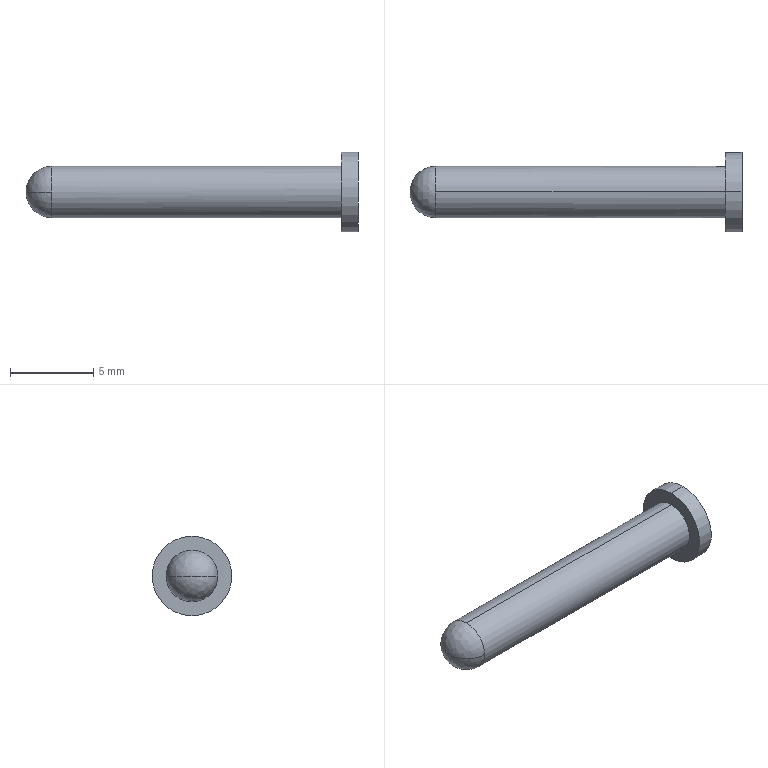Part | STEP file | 0217_Z_PJL8-10-2 | 1 solid | 8 faces | box 20 x 4.8 x 4.8 mm | volume 157.602 mm3 | cylinder 4 | spline 2 | plane 2 | commonest cylinder face diameters 3.1 x2 4.8 x2
STEP:
#1=CARTESIAN_POINT('',(0.,0.,0.));
#2=DIRECTION('',(0.,0.,1.));
#3=DIRECTION('',(1.,0.,0.));
#4=AXIS2_PLACEMENT_3D('',#1,#2,#3);
#5=CARTESIAN_POINT('',(-8.45,-1.55,0.));
#6=VERTEX_POINT('',#5);
#7=CARTESIAN_POINT('',(-8.45,0.,-1.55));
#8=VERTEX_POINT('',#7);
#9=CARTESIAN_POINT('',(-8.45,0.,0.));
#10=DIRECTION('',(1.,0.,0.));
#11=DIRECTION('',(0.,0.,-1.));
#12=AXIS2_PLACEMENT_3D('',#9,#10,#11);
#13=CIRCLE('',#12,1.55);
#14=CARTESIAN_POINT('',(-8.45,-1.55,0.));
#15=CARTESIAN_POINT('',(-8.45,-1.55,-3.1));
#16=CARTESIAN_POINT('',(-8.45,1.55,-3.1));
#17=CARTESIAN_POINT('',(-8.45,1.55,0.));
#18=CARTESIAN_POINT('',(-9.358,-1.55,0.));
#19=CARTESIAN_POINT('',(-9.358,-1.55,-3.1));
#20=CARTESIAN_POINT('',(-9.358,1.55,-3.1));
#21=CARTESIAN_POINT('',(-9.358,1.55,0.));
#22=CARTESIAN_POINT('',(-10.,-0.908,0.));
#23=CARTESIAN_POINT('',(-10.,-0.908,-1.816));
#24=CARTESIAN_POINT('',(-10.,0.908,-1.816));
#25=CARTESIAN_POINT('',(-10.,0.908,0.));
#26=CARTESIAN_POINT('',(-10.,0.,0.));
#27=CARTESIAN_POINT('',(-10.,0.,0.));
#28=CARTESIAN_POINT('',(-10.,0.,0.));
#29=CARTESIAN_POINT('',(-10.,0.,0.));
#30=(BOUNDED_SURFACE()B_SPLINE_SURFACE(3,3,((#14,#15,#16,#17),(#18,#19,#20,#21),(#22,#23,#24,#25),(#26,#27,#28,#29)),.UNSPECIFIED.,.F.,.F.,.F.)B_SPLINE_SURFACE_WITH_KNOTS((4,4),(4,4),(0.,1.),(0.,1.),.PIECEWISE_BEZIER_KNOTS.)GEOMETRIC_REPRESENTATION_ITEM()RATIONAL_B_SPLINE_SURFACE(((1.,0.3333,0.3333,1.),(0.8047,0.2682,0.2682,0.8047),(0.8047,0.2682,0.2682,0.8047),(1.,0.3333,0.3333,1.)))REPRESENTATION_ITEM('')SURFACE());
#31=CARTESIAN_POINT('',(0.,0.));
#32=CARTESIAN_POINT('',(0.,0.0119));
#33=CARTESIAN_POINT('',(0.,0.03485));
#34=CARTESIAN_POINT('',(0.,0.06707));
#35=CARTESIAN_POINT('',(0.,0.09736));
#36=CARTESIAN_POINT('',(0.,0.126));
#37=CARTESIAN_POINT('',(0.,0.1531));
#38=CARTESIAN_POINT('',(0.,0.1789));
#39=CARTESIAN_POINT('',(0.,0.2035));
#40=CARTESIAN_POINT('',(0.,0.2271));
#41=CARTESIAN_POINT('',(0.,0.2499));
#42=CARTESIAN_POINT('',(0.,0.2718));
#43=CARTESIAN_POINT('',(0.,0.293));
#44=CARTESIAN_POINT('',(0.,0.3136));
#45=CARTESIAN_POINT('',(0.,0.3337));
#46=CARTESIAN_POINT('',(0.,0.3533));
#47=CARTESIAN_POINT('',(0.,0.3724));
#48=CARTESIAN_POINT('',(0.,0.3913));
#49=CARTESIAN_POINT('',(0.,0.4098));
#50=CARTESIAN_POINT('',(0.,0.4281));
#51=CARTESIAN_POINT('',(0.,0.4463));
#52=CARTESIAN_POINT('',(0.,0.4643));
#53=CARTESIAN_POINT('',(0.,0.4822));
#54=CARTESIAN_POINT('',(0.,0.494));
#55=CARTESIAN_POINT('',(0.,0.5));
#56=B_SPLINE_CURVE_WITH_KNOTS('',3,(#31,#32,#33,#34,#35,#36,#37,#38,#39,#40,#41,#42,#43,#44,#45,#46,#47,#48,#49,#50,#51,#52,#53,#54,#55),.UNSPECIFIED.,.F.,.F.,(4,1,1,1,1,1,1,1,1,1,1,1,1,1,1,1,1,1,1,1,1,1,4),(4.712,4.784,4.855,4.927,4.998,5.069,5.141,5.212,5.284,5.355,5.426,5.498,5.569,5.641,5.712,5.783,5.855,5.926,5.998,6.069,6.14,6.212,6.283),.QUASI_UNIFORM_KNOTS.);
#57=(GEOMETRIC_REPRESENTATION_CONTEXT(2)PARAMETRIC_REPRESENTATION_CONTEXT()REPRESENTATION_CONTEXT('',''));
#58=DEFINITIONAL_REPRESENTATION('',(#56),#57);
#59=PCURVE('',#30,#58);
#60=CARTESIAN_POINT('',(0.275,0.,0.));
#61=DIRECTION('',(1.,0.,0.));
#62=DIRECTION('',(0.,0.,-1.));
#63=AXIS2_PLACEMENT_3D('',#60,#61,#62);
#64=CYLINDRICAL_SURFACE('',#63,1.55);
#65=CARTESIAN_POINT('',(0.,-8.725));
#66=DIRECTION('',(1.,0.));
#67=VECTOR('',#66,1.);
#68=LINE('',#65,#67);
#69=(GEOMETRIC_REPRESENTATION_CONTEXT(2)PARAMETRIC_REPRESENTATION_CONTEXT()REPRESENTATION_CONTEXT('',''));
#70=DEFINITIONAL_REPRESENTATION('',(#68),#69);
#71=PCURVE('',#64,#70);
#72=SURFACE_CURVE('',#13,(#59,#71),.PCURVE_S1.);
#73=EDGE_CURVE('',#6,#8,#72,.T.);
#74=ORIENTED_EDGE('',*,*,#73,.F.);
#75=CARTESIAN_POINT('',(-10.,0.,0.));
#76=VERTEX_POINT('',#75);
#77=CARTESIAN_POINT('',(-8.45,0.,0.));
#78=DIRECTION('',(0.,0.,-1.));
#79=DIRECTION('',(1.,0.,0.));
#80=AXIS2_PLACEMENT_3D('',#77,#78,#79);
#81=CIRCLE('',#80,1.55);
#82=CARTESIAN_POINT('',(0.,0.));
#83=CARTESIAN_POINT('',(0.01683,0.));
#84=CARTESIAN_POINT('',(0.04999,0.));
#85=CARTESIAN_POINT('',(0.09843,0.));
#86=CARTESIAN_POINT('',(0.1457,0.));
#87=CARTESIAN_POINT('',(0.192,0.));
#88=CARTESIAN_POINT('',(0.2375,0.));
#89=CARTESIAN_POINT('',(0.2823,0.));
#90=CARTESIAN_POINT('',(0.3265,0.));
#91=CARTESIAN_POINT('',(0.3703,0.));
#92=CARTESIAN_POINT('',(0.4137,0.));
#93=CARTESIAN_POINT('',(0.4569,0.));
#94=CARTESIAN_POINT('',(0.5,0.));
#95=CARTESIAN_POINT('',(0.5431,0.));
#96=CARTESIAN_POINT('',(0.5863,0.));
#97=CARTESIAN_POINT('',(0.6297,0.));
#98=CARTESIAN_POINT('',(0.6735,0.));
#99=CARTESIAN_POINT('',(0.7177,0.));
#100=CARTESIAN_POINT('',(0.7625,0.));
#101=CARTESIAN_POINT('',(0.808,0.));
#102=CARTESIAN_POINT('',(0.8543,0.));
#103=CARTESIAN_POINT('',(0.9016,0.));
#104=CARTESIAN_POINT('',(0.95,0.));
#105=CARTESIAN_POINT('',(0.9832,0.));
#106=CARTESIAN_POINT('',(1.,0.));
#107=B_SPLINE_CURVE_WITH_KNOTS('',3,(#82,#83,#84,#85,#86,#87,#88,#89,#90,#91,#92,#93,#94,#95,#96,#97,#98,#99,#100,#101,#102,#103,#104,#105,#106),.UNSPECIFIED.,.F.,.F.,(4,1,1,1,1,1,1,1,1,1,1,1,1,1,1,1,1,1,1,1,1,1,4),(1.571,1.642,1.714,1.785,1.856,1.928,1.999,2.071,2.142,2.213,2.285,2.356,2.428,2.499,2.57,2.642,2.713,2.785,2.856,2.927,2.999,3.07,3.142),.QUASI_UNIFORM_KNOTS.);
#108=(GEOMETRIC_REPRESENTATION_CONTEXT(2)PARAMETRIC_REPRESENTATION_CONTEXT()REPRESENTATION_CONTEXT('',''));
#109=DEFINITIONAL_REPRESENTATION('',(#107),#108);
#110=PCURVE('',#30,#109);
#111=CARTESIAN_POINT('',(-8.45,1.55,0.));
#112=CARTESIAN_POINT('',(-8.45,1.55,3.1));
#113=CARTESIAN_POINT('',(-8.45,-1.55,3.1));
#114=CARTESIAN_POINT('',(-8.45,-1.55,0.));
#115=CARTESIAN_POINT('',(-9.358,1.55,0.));
#116=CARTESIAN_POINT('',(-9.358,1.55,3.1));
#117=CARTESIAN_POINT('',(-9.358,-1.55,3.1));
#118=CARTESIAN_POINT('',(-9.358,-1.55,0.));
#119=CARTESIAN_POINT('',(-10.,0.908,0.));
#120=CARTESIAN_POINT('',(-10.,0.908,1.816));
#121=CARTESIAN_POINT('',(-10.,-0.908,1.816));
#122=CARTESIAN_POINT('',(-10.,-0.908,0.));
#123=CARTESIAN_POINT('',(-10.,0.,0.));
#124=CARTESIAN_POINT('',(-10.,0.,0.));
#125=CARTESIAN_POINT('',(-10.,0.,0.));
#126=CARTESIAN_POINT('',(-10.,0.,0.));
#127=(BOUNDED_SURFACE()B_SPLINE_SURFACE(3,3,((#111,#112,#113,#114),(#115,#116,#117,#118),(#119,#120,#121,#122),(#123,#124,#125,#126)),.UNSPECIFIED.,.F.,.F.,.F.)B_SPLINE_SURFACE_WITH_KNOTS((4,4),(4,4),(0.,1.),(0.,1.),.PIECEWISE_BEZIER_KNOTS.)GEOMETRIC_REPRESENTATION_ITEM()RATIONAL_B_SPLINE_SURFACE(((1.,0.3333,0.3333,1.),(0.8047,0.2682,0.2682,0.8047),(0.8047,0.2682,0.2682,0.8047),(1.,0.3333,0.3333,1.)))REPRESENTATION_ITEM('')SURFACE());
#128=CARTESIAN_POINT('',(0.,1.));
#129=CARTESIAN_POINT('',(0.01683,1.));
#130=CARTESIAN_POINT('',(0.04999,1.));
#131=CARTESIAN_POINT('',(0.09843,1.));
#132=CARTESIAN_POINT('',(0.1457,1.));
#133=CARTESIAN_POINT('',(0.192,1.));
#134=CARTESIAN_POINT('',(0.2375,1.));
#135=CARTESIAN_POINT('',(0.2823,1.));
#136=CARTESIAN_POINT('',(0.3265,1.));
#137=CARTESIAN_POINT('',(0.3703,1.));
#138=CARTESIAN_POINT('',(0.4137,1.));
#139=CARTESIAN_POINT('',(0.4569,1.));
#140=CARTESIAN_POINT('',(0.5,1.));
#141=CARTESIAN_POINT('',(0.5431,1.));
#142=CARTESIAN_POINT('',(0.5863,1.));
#143=CARTESIAN_POINT('',(0.6297,1.));
#144=CARTESIAN_POINT('',(0.6735,1.));
#145=CARTESIAN_POINT('',(0.7177,1.));
#146=CARTESIAN_POINT('',(0.7625,1.));
#147=CARTESIAN_POINT('',(0.808,1.));
#148=CARTESIAN_POINT('',(0.8543,1.));
#149=CARTESIAN_POINT('',(0.9016,1.));
#150=CARTESIAN_POINT('',(0.95,1.));
#151=CARTESIAN_POINT('',(0.9832,1.));
#152=CARTESIAN_POINT('',(1.,1.));
#153=B_SPLINE_CURVE_WITH_KNOTS('',3,(#128,#129,#130,#131,#132,#133,#134,#135,#136,#137,#138,#139,#140,#141,#142,#143,#144,#145,#146,#147,#148,#149,#150,#151,#152),.UNSPECIFIED.,.F.,.F.,(4,1,1,1,1,1,1,1,1,1,1,1,1,1,1,1,1,1,1,1,1,1,4),(1.571,1.642,1.714,1.785,1.856,1.928,1.999,2.071,2.142,2.213,2.285,2.356,2.428,2.499,2.57,2.642,2.713,2.785,2.856,2.927,2.999,3.07,3.142),.QUASI_UNIFORM_KNOTS.);
#154=(GEOMETRIC_REPRESENTATION_CONTEXT(2)PARAMETRIC_REPRESENTATION_CONTEXT()REPRESENTATION_CONTEXT('',''));
#155=DEFINITIONAL_REPRESENTATION('',(#153),#154);
#156=PCURVE('',#127,#155);
#157=SURFACE_CURVE('',#81,(#110,#156),.PCURVE_S1.);
#158=EDGE_CURVE('',#6,#76,#157,.T.);
#159=ORIENTED_EDGE('',*,*,#158,.T.);
#160=CARTESIAN_POINT('',(-8.45,1.55,0.));
#161=VERTEX_POINT('',#160);
#162=CARTESIAN_POINT('',(-8.45,0.,0.));
#163=DIRECTION('',(0.,0.,1.));
#164=DIRECTION('',(1.,0.,0.));
#165=AXIS2_PLACEMENT_3D('',#162,#163,#164);
#166=CIRCLE('',#165,1.55);
#167=CARTESIAN_POINT('',(0.,1.));
#168=CARTESIAN_POINT('',(0.01683,1.));
#169=CARTESIAN_POINT('',(0.04999,1.));
#170=CARTESIAN_POINT('',(0.09843,1.));
#171=CARTESIAN_POINT('',(0.1457,1.));
#172=CARTESIAN_POINT('',(0.192,1.));
#173=CARTESIAN_POINT('',(0.2375,1.));
#174=CARTESIAN_POINT('',(0.2823,1.));
#175=CARTESIAN_POINT('',(0.3265,1.));
#176=CARTESIAN_POINT('',(0.3703,1.));
#177=CARTESIAN_POINT('',(0.4137,1.));
#178=CARTESIAN_POINT('',(0.4569,1.));
#179=CARTESIAN_POINT('',(0.5,1.));
#180=CARTESIAN_POINT('',(0.5431,1.));
#181=CARTESIAN_POINT('',(0.5863,1.));
#182=CARTESIAN_POINT('',(0.6297,1.));
#183=CARTESIAN_POINT('',(0.6735,1.));
#184=CARTESIAN_POINT('',(0.7177,1.));
#185=CARTESIAN_POINT('',(0.7625,1.));
#186=CARTESIAN_POINT('',(0.808,1.));
#187=CARTESIAN_POINT('',(0.8543,1.));
#188=CARTESIAN_POINT('',(0.9016,1.));
#189=CARTESIAN_POINT('',(0.95,1.));
#190=CARTESIAN_POINT('',(0.9832,1.));
#191=CARTESIAN_POINT('',(1.,1.));
#192=B_SPLINE_CURVE_WITH_KNOTS('',3,(#167,#168,#169,#170,#171,#172,#173,#174,#175,#176,#177,#178,#179,#180,#181,#182,#183,#184,#185,#186,#187,#188,#189,#190,#191),.UNSPECIFIED.,.F.,.F.,(4,1,1,1,1,1,1,1,1,1,1,1,1,1,1,1,1,1,1,1,1,1,4),(1.571,1.642,1.714,1.785,1.856,1.928,1.999,2.071,2.142,2.213,2.285,2.356,2.428,2.499,2.57,2.642,2.713,2.785,2.856,2.927,2.999,3.07,3.142),.QUASI_UNIFORM_KNOTS.);
#193=(GEOMETRIC_REPRESENTATION_CONTEXT(2)PARAMETRIC_REPRESENTATION_CONTEXT()REPRESENTATION_CONTEXT('',''));
#194=DEFINITIONAL_REPRESENTATION('',(#192),#193);
#195=PCURVE('',#30,#194);
#196=CARTESIAN_POINT('',(0.,0.));
#197=CARTESIAN_POINT('',(0.01683,0.));
#198=CARTESIAN_POINT('',(0.04999,0.));
#199=CARTESIAN_POINT('',(0.09843,0.));
#200=CARTESIAN_POINT('',(0.1457,0.));
#201=CARTESIAN_POINT('',(0.192,0.));
#202=CARTESIAN_POINT('',(0.2375,0.));
#203=CARTESIAN_POINT('',(0.2823,0.));
#204=CARTESIAN_POINT('',(0.3265,0.));
#205=CARTESIAN_POINT('',(0.3703,0.));
#206=CARTESIAN_POINT('',(0.4137,0.));
#207=CARTESIAN_POINT('',(0.4569,0.));
#208=CARTESIAN_POINT('',(0.5,0.));
#209=CARTESIAN_POINT('',(0.5431,0.));
#210=CARTESIAN_POINT('',(0.5863,0.));
#211=CARTESIAN_POINT('',(0.6297,0.));
#212=CARTESIAN_POINT('',(0.6735,0.));
#213=CARTESIAN_POINT('',(0.7177,0.));
#214=CARTESIAN_POINT('',(0.7625,0.));
#215=CARTESIAN_POINT('',(0.808,0.));
#216=CARTESIAN_POINT('',(0.8543,0.));
#217=CARTESIAN_POINT('',(0.9016,0.));
#218=CARTESIAN_POINT('',(0.95,0.));
#219=CARTESIAN_POINT('',(0.9832,0.));
#220=CARTESIAN_POINT('',(1.,0.));
#221=B_SPLINE_CURVE_WITH_KNOTS('',3,(#196,#197,#198,#199,#200,#201,#202,#203,#204,#205,#206,#207,#208,#209,#210,#211,#212,#213,#214,#215,#216,#217,#218,#219,#220),.UNSPECIFIED.,.F.,.F.,(4,1,1,1,1,1,1,1,1,1,1,1,1,1,1,1,1,1,1,1,1,1,4),(1.571,1.642,1.714,1.785,1.856,1.928,1.999,2.071,2.142,2.213,2.285,2.356,2.428,2.499,2.57,2.642,2.713,2.785,2.856,2.927,2.999,3.07,3.142),.QUASI_UNIFORM_KNOTS.);
#222=(GEOMETRIC_REPRESENTATION_CONTEXT(2)PARAMETRIC_REPRESENTATION_CONTEXT()REPRESENTATION_CONTEXT('',''));
#223=DEFINITIONAL_REPRESENTATION('',(#221),#222);
#224=PCURVE('',#127,#223);
#225=SURFACE_CURVE('',#166,(#195,#224),.PCURVE_S1.);
#226=EDGE_CURVE('',#161,#76,#225,.T.);
#227=ORIENTED_EDGE('',*,*,#226,.F.);
#228=CARTESIAN_POINT('',(-8.45,0.,0.));
#229=DIRECTION('',(1.,0.,0.));
#230=DIRECTION('',(0.,0.,-1.));
#231=AXIS2_PLACEMENT_3D('',#228,#229,#230);
#232=CIRCLE('',#231,1.55);
#233=CARTESIAN_POINT('',(0.,0.5));
#234=CARTESIAN_POINT('',(0.,0.506));
#235=CARTESIAN_POINT('',(0.,0.5178));
#236=CARTESIAN_POINT('',(0.,0.5357));
#237=CARTESIAN_POINT('',(0.,0.5537));
#238=CARTESIAN_POINT('',(0.,0.5719));
#239=CARTESIAN_POINT('',(0.,0.5902));
#240=CARTESIAN_POINT('',(0.,0.6087));
#241=CARTESIAN_POINT('',(0.,0.6276));
#242=CARTESIAN_POINT('',(0.,0.6467));
#243=CARTESIAN_POINT('',(0.,0.6663));
#244=CARTESIAN_POINT('',(0.,0.6864));
#245=CARTESIAN_POINT('',(0.,0.707));
#246=CARTESIAN_POINT('',(0.,0.7282));
#247=CARTESIAN_POINT('',(0.,0.7501));
#248=CARTESIAN_POINT('',(0.,0.7729));
#249=CARTESIAN_POINT('',(0.,0.7965));
#250=CARTESIAN_POINT('',(0.,0.8211));
#251=CARTESIAN_POINT('',(0.,0.8469));
#252=CARTESIAN_POINT('',(0.,0.874));
#253=CARTESIAN_POINT('',(0.,0.9026));
#254=CARTESIAN_POINT('',(0.,0.9329));
#255=CARTESIAN_POINT('',(0.,0.9651));
#256=CARTESIAN_POINT('',(0.,0.9881));
#257=CARTESIAN_POINT('',(0.,1.));
#258=B_SPLINE_CURVE_WITH_KNOTS('',3,(#233,#234,#235,#236,#237,#238,#239,#240,#241,#242,#243,#244,#245,#246,#247,#248,#249,#250,#251,#252,#253,#254,#255,#256,#257),.UNSPECIFIED.,.F.,.F.,(4,1,1,1,1,1,1,1,1,1,1,1,1,1,1,1,1,1,1,1,1,1,4),(0.,0.0714,0.1428,0.2142,0.2856,0.357,0.4284,0.4998,0.5712,0.6426,0.714,0.7854,0.8568,0.9282,0.9996,1.071,1.142,1.214,1.285,1.357,1.428,1.499,1.571),.QUASI_UNIFORM_KNOTS.);
#259=(GEOMETRIC_REPRESENTATION_CONTEXT(2)PARAMETRIC_REPRESENTATION_CONTEXT()REPRESENTATION_CONTEXT('',''));
#260=DEFINITIONAL_REPRESENTATION('',(#258),#259);
#261=PCURVE('',#30,#260);
#262=CARTESIAN_POINT('',(0.275,0.,0.));
#263=DIRECTION('',(1.,0.,0.));
#264=DIRECTION('',(0.,0.,-1.));
#265=AXIS2_PLACEMENT_3D('',#262,#263,#264);
#266=CYLINDRICAL_SURFACE('',#265,1.55);
#267=CARTESIAN_POINT('',(0.,-8.725));
#268=DIRECTION('',(1.,0.));
#269=VECTOR('',#268,1.);
#270=LINE('',#267,#269);
#271=(GEOMETRIC_REPRESENTATION_CONTEXT(2)PARAMETRIC_REPRESENTATION_CONTEXT()REPRESENTATION_CONTEXT('',''));
#272=DEFINITIONAL_REPRESENTATION('',(#270),#271);
#273=PCURVE('',#266,#272);
#274=SURFACE_CURVE('',#232,(#261,#273),.PCURVE_S1.);
#275=EDGE_CURVE('',#8,#161,#274,.T.);
#276=ORIENTED_EDGE('',*,*,#275,.F.);
#277=EDGE_LOOP('',(#74,#159,#227,#276));
#278=FACE_BOUND('',#277,.T.);
#279=ADVANCED_FACE('',(#278),#30,.T.);
#280=ORIENTED_EDGE('',*,*,#275,.T.);
#281=CARTESIAN_POINT('',(-8.45,0.,1.55));
#282=VERTEX_POINT('',#281);
#283=CARTESIAN_POINT('',(-8.45,0.,0.));
#284=DIRECTION('',(1.,0.,0.));
#285=DIRECTION('',(0.,0.,-1.));
#286=AXIS2_PLACEMENT_3D('',#283,#284,#285);
#287=CIRCLE('',#286,1.55);
#288=CARTESIAN_POINT('',(0.,-8.725));
#289=DIRECTION('',(1.,0.));
#290=VECTOR('',#289,1.);
#291=LINE('',#288,#290);
#292=(GEOMETRIC_REPRESENTATION_CONTEXT(2)PARAMETRIC_REPRESENTATION_CONTEXT()REPRESENTATION_CONTEXT('',''));
#293=DEFINITIONAL_REPRESENTATION('',(#291),#292);
#294=PCURVE('',#266,#293);
#295=CARTESIAN_POINT('',(0.,0.));
#296=CARTESIAN_POINT('',(0.,0.0119));
#297=CARTESIAN_POINT('',(0.,0.03485));
#298=CARTESIAN_POINT('',(0.,0.06707));
#299=CARTESIAN_POINT('',(0.,0.09736));
#300=CARTESIAN_POINT('',(0.,0.126));
#301=CARTESIAN_POINT('',(0.,0.1531));
#302=CARTESIAN_POINT('',(0.,0.1789));
#303=CARTESIAN_POINT('',(0.,0.2035));
#304=CARTESIAN_POINT('',(0.,0.2271));
#305=CARTESIAN_POINT('',(0.,0.2499));
#306=CARTESIAN_POINT('',(0.,0.2718));
#307=CARTESIAN_POINT('',(0.,0.293));
#308=CARTESIAN_POINT('',(0.,0.3136));
#309=CARTESIAN_POINT('',(0.,0.3337));
#310=CARTESIAN_POINT('',(0.,0.3533));
#311=CARTESIAN_POINT('',(0.,0.3724));
#312=CARTESIAN_POINT('',(0.,0.3913));
#313=CARTESIAN_POINT('',(0.,0.4098));
#314=CARTESIAN_POINT('',(0.,0.4281));
#315=CARTESIAN_POINT('',(0.,0.4463));
#316=CARTESIAN_POINT('',(0.,0.4643));
#317=CARTESIAN_POINT('',(0.,0.4822));
#318=CARTESIAN_POINT('',(0.,0.494));
#319=CARTESIAN_POINT('',(0.,0.5));
#320=B_SPLINE_CURVE_WITH_KNOTS('',3,(#295,#296,#297,#298,#299,#300,#301,#302,#303,#304,#305,#306,#307,#308,#309,#310,#311,#312,#313,#314,#315,#316,#317,#318,#319),.UNSPECIFIED.,.F.,.F.,(4,1,1,1,1,1,1,1,1,1,1,1,1,1,1,1,1,1,1,1,1,1,4),(1.571,1.642,1.714,1.785,1.856,1.928,1.999,2.071,2.142,2.213,2.285,2.356,2.428,2.499,2.57,2.642,2.713,2.785,2.856,2.927,2.999,3.07,3.142),.QUASI_UNIFORM_KNOTS.);
#321=(GEOMETRIC_REPRESENTATION_CONTEXT(2)PARAMETRIC_REPRESENTATION_CONTEXT()REPRESENTATION_CONTEXT('',''));
#322=DEFINITIONAL_REPRESENTATION('',(#320),#321);
#323=PCURVE('',#127,#322);
#324=SURFACE_CURVE('',#287,(#294,#323),.PCURVE_S1.);
#325=EDGE_CURVE('',#161,#282,#324,.T.);
#326=ORIENTED_EDGE('',*,*,#325,.T.);
#327=CARTESIAN_POINT('',(9.,0.,1.55));
#328=VERTEX_POINT('',#327);
#329=CARTESIAN_POINT('',(0.275,0.,1.55));
#330=DIRECTION('',(1.,0.,0.));
#331=VECTOR('',#330,1.);
#332=LINE('',#329,#331);
#333=CARTESIAN_POINT('',(3.142,0.));
#334=DIRECTION('',(0.,1.));
#335=VECTOR('',#334,1.);
#336=LINE('',#333,#335);
#337=(GEOMETRIC_REPRESENTATION_CONTEXT(2)PARAMETRIC_REPRESENTATION_CONTEXT()REPRESENTATION_CONTEXT('',''));
#338=DEFINITIONAL_REPRESENTATION('',(#336),#337);
#339=PCURVE('',#266,#338);
#340=CARTESIAN_POINT('',(3.142,0.));
#341=DIRECTION('',(0.,1.));
#342=VECTOR('',#341,1.);
#343=LINE('',#340,#342);
#344=(GEOMETRIC_REPRESENTATION_CONTEXT(2)PARAMETRIC_REPRESENTATION_CONTEXT()REPRESENTATION_CONTEXT('',''));
#345=DEFINITIONAL_REPRESENTATION('',(#343),#344);
#346=PCURVE('',#64,#345);
#347=SURFACE_CURVE('',#332,(#339,#346),.PCURVE_S1.);
#348=EDGE_CURVE('',#282,#328,#347,.T.);
#349=ORIENTED_EDGE('',*,*,#348,.T.);
#350=CARTESIAN_POINT('',(9.,0.,-1.55));
#351=VERTEX_POINT('',#350);
#352=CARTESIAN_POINT('',(9.,0.,0.));
#353=DIRECTION('',(-1.,0.,0.));
#354=DIRECTION('',(0.,0.,-1.));
#355=AXIS2_PLACEMENT_3D('',#352,#353,#354);
#356=CIRCLE('',#355,1.55);
#357=CARTESIAN_POINT('',(6.283,8.725));
#358=DIRECTION('',(-1.,0.));
#359=VECTOR('',#358,1.);
#360=LINE('',#357,#359);
#361=(GEOMETRIC_REPRESENTATION_CONTEXT(2)PARAMETRIC_REPRESENTATION_CONTEXT()REPRESENTATION_CONTEXT('',''));
#362=DEFINITIONAL_REPRESENTATION('',(#360),#361);
#363=PCURVE('',#266,#362);
#364=CARTESIAN_POINT('',(9.,1.975,0.));
#365=DIRECTION('',(-1.,0.,0.));
#366=DIRECTION('',(0.,0.,1.));
#367=AXIS2_PLACEMENT_3D('',#364,#365,#366);
#368=PLANE('',#367);
#369=CARTESIAN_POINT('',(0.,-1.975));
#370=DIRECTION('',(-1.,0.));
#371=AXIS2_PLACEMENT_2D('',#369,#370);
#372=CIRCLE('',#371,1.55);
#373=(GEOMETRIC_REPRESENTATION_CONTEXT(2)PARAMETRIC_REPRESENTATION_CONTEXT()REPRESENTATION_CONTEXT('',''));
#374=DEFINITIONAL_REPRESENTATION('',(#372),#373);
#375=PCURVE('',#368,#374);
#376=SURFACE_CURVE('',#356,(#363,#375),.PCURVE_S1.);
#377=EDGE_CURVE('',#328,#351,#376,.T.);
#378=ORIENTED_EDGE('',*,*,#377,.T.);
#379=CARTESIAN_POINT('',(0.275,0.,-1.55));
#380=DIRECTION('',(1.,0.,0.));
#381=VECTOR('',#380,1.);
#382=LINE('',#379,#381);
#383=CARTESIAN_POINT('',(0.,0.));
#384=DIRECTION('',(0.,1.));
#385=VECTOR('',#384,1.);
#386=LINE('',#383,#385);
#387=(GEOMETRIC_REPRESENTATION_CONTEXT(2)PARAMETRIC_REPRESENTATION_CONTEXT()REPRESENTATION_CONTEXT('',''));
#388=DEFINITIONAL_REPRESENTATION('',(#386),#387);
#389=PCURVE('',#266,#388);
#390=CARTESIAN_POINT('',(6.283,0.));
#391=DIRECTION('',(0.,1.));
#392=VECTOR('',#391,1.);
#393=LINE('',#390,#392);
#394=(GEOMETRIC_REPRESENTATION_CONTEXT(2)PARAMETRIC_REPRESENTATION_CONTEXT()REPRESENTATION_CONTEXT('',''));
#395=DEFINITIONAL_REPRESENTATION('',(#393),#394);
#396=PCURVE('',#64,#395);
#397=SURFACE_CURVE('',#382,(#389,#396),.PCURVE_S1.);
#398=EDGE_CURVE('',#8,#351,#397,.T.);
#399=ORIENTED_EDGE('',*,*,#398,.F.);
#400=EDGE_LOOP('',(#280,#326,#349,#378,#399));
#401=FACE_BOUND('',#400,.T.);
#402=ADVANCED_FACE('',(#401),#266,.T.);
#403=CARTESIAN_POINT('',(9.,0.,2.4));
#404=VERTEX_POINT('',#403);
#405=CARTESIAN_POINT('',(9.,0.,-2.4));
#406=VERTEX_POINT('',#405);
#407=CARTESIAN_POINT('',(9.,0.,0.));
#408=DIRECTION('',(-1.,0.,0.));
#409=DIRECTION('',(0.,0.,-1.));
#410=AXIS2_PLACEMENT_3D('',#407,#408,#409);
#411=CIRCLE('',#410,2.4);
#412=CARTESIAN_POINT('',(9.5,0.,0.));
#413=DIRECTION('',(1.,0.,0.));
#414=DIRECTION('',(0.,0.,-1.));
#415=AXIS2_PLACEMENT_3D('',#412,#413,#414);
#416=CYLINDRICAL_SURFACE('',#415,2.4);
#417=CARTESIAN_POINT('',(6.283,-0.5));
#418=DIRECTION('',(-1.,0.));
#419=VECTOR('',#418,1.);
#420=LINE('',#417,#419);
#421=(GEOMETRIC_REPRESENTATION_CONTEXT(2)PARAMETRIC_REPRESENTATION_CONTEXT()REPRESENTATION_CONTEXT('',''));
#422=DEFINITIONAL_REPRESENTATION('',(#420),#421);
#423=PCURVE('',#416,#422);
#424=CARTESIAN_POINT('',(0.,-1.975));
#425=DIRECTION('',(-1.,0.));
#426=AXIS2_PLACEMENT_2D('',#424,#425);
#427=CIRCLE('',#426,2.4);
#428=(GEOMETRIC_REPRESENTATION_CONTEXT(2)PARAMETRIC_REPRESENTATION_CONTEXT()REPRESENTATION_CONTEXT('',''));
#429=DEFINITIONAL_REPRESENTATION('',(#427),#428);
#430=PCURVE('',#368,#429);
#431=SURFACE_CURVE('',#411,(#423,#430),.PCURVE_S1.);
#432=EDGE_CURVE('',#404,#406,#431,.T.);
#433=ORIENTED_EDGE('',*,*,#432,.F.);
#434=CARTESIAN_POINT('',(10.,0.,2.4));
#435=VERTEX_POINT('',#434);
#436=CARTESIAN_POINT('',(9.5,0.,2.4));
#437=DIRECTION('',(1.,0.,0.));
#438=VECTOR('',#437,1.);
#439=LINE('',#436,#438);
#440=CARTESIAN_POINT('',(3.142,0.));
#441=DIRECTION('',(0.,1.));
#442=VECTOR('',#441,1.);
#443=LINE('',#440,#442);
#444=(GEOMETRIC_REPRESENTATION_CONTEXT(2)PARAMETRIC_REPRESENTATION_CONTEXT()REPRESENTATION_CONTEXT('',''));
#445=DEFINITIONAL_REPRESENTATION('',(#443),#444);
#446=PCURVE('',#416,#445);
#447=CARTESIAN_POINT('',(9.5,0.,0.));
#448=DIRECTION('',(1.,0.,0.));
#449=DIRECTION('',(0.,0.,-1.));
#450=AXIS2_PLACEMENT_3D('',#447,#448,#449);
#451=CYLINDRICAL_SURFACE('',#450,2.4);
#452=CARTESIAN_POINT('',(3.142,0.));
#453=DIRECTION('',(0.,1.));
#454=VECTOR('',#453,1.);
#455=LINE('',#452,#454);
#456=(GEOMETRIC_REPRESENTATION_CONTEXT(2)PARAMETRIC_REPRESENTATION_CONTEXT()REPRESENTATION_CONTEXT('',''));
#457=DEFINITIONAL_REPRESENTATION('',(#455),#456);
#458=PCURVE('',#451,#457);
#459=SURFACE_CURVE('',#439,(#446,#458),.PCURVE_S1.);
#460=EDGE_CURVE('',#404,#435,#459,.T.);
#461=ORIENTED_EDGE('',*,*,#460,.T.);
#462=CARTESIAN_POINT('',(10.,0.,-2.4));
#463=VERTEX_POINT('',#462);
#464=CARTESIAN_POINT('',(10.,0.,0.));
#465=DIRECTION('',(-1.,0.,0.));
#466=DIRECTION('',(0.,0.,-1.));
#467=AXIS2_PLACEMENT_3D('',#464,#465,#466);
#468=CIRCLE('',#467,2.4);
#469=CARTESIAN_POINT('',(6.283,0.5));
#470=DIRECTION('',(-1.,0.));
#471=VECTOR('',#470,1.);
#472=LINE('',#469,#471);
#473=(GEOMETRIC_REPRESENTATION_CONTEXT(2)PARAMETRIC_REPRESENTATION_CONTEXT()REPRESENTATION_CONTEXT('',''));
#474=DEFINITIONAL_REPRESENTATION('',(#472),#473);
#475=PCURVE('',#416,#474);
#476=CARTESIAN_POINT('',(10.,1.2,0.));
#477=DIRECTION('',(1.,0.,0.));
#478=DIRECTION('',(0.,0.,-1.));
#479=AXIS2_PLACEMENT_3D('',#476,#477,#478);
#480=PLANE('',#479);
#481=CARTESIAN_POINT('',(2.4,-1.2));
#482=CARTESIAN_POINT('',(2.4,-5.357));
#483=CARTESIAN_POINT('',(-1.2,-3.278));
#484=CARTESIAN_POINT('',(-4.8,-1.2));
#485=CARTESIAN_POINT('',(-1.2,0.8785));
#486=CARTESIAN_POINT('',(2.4,2.957));
#487=CARTESIAN_POINT('',(2.4,-1.2));
#488=(BOUNDED_CURVE()B_SPLINE_CURVE(2,(#481,#482,#483,#484,#485,#486,#487),.UNSPECIFIED.,.T.,.F.)B_SPLINE_CURVE_WITH_KNOTS((1,2,2,2,2,1),(-2.094,0.,2.094,4.189,6.283,8.378),.UNSPECIFIED.)CURVE()GEOMETRIC_REPRESENTATION_ITEM()RATIONAL_B_SPLINE_CURVE((1.,0.5,1.,0.5,1.,0.5,1.))REPRESENTATION_ITEM(''));
#489=(GEOMETRIC_REPRESENTATION_CONTEXT(2)PARAMETRIC_REPRESENTATION_CONTEXT()REPRESENTATION_CONTEXT('',''));
#490=DEFINITIONAL_REPRESENTATION('',(#488),#489);
#491=PCURVE('',#480,#490);
#492=SURFACE_CURVE('',#468,(#475,#491),.PCURVE_S1.);
#493=EDGE_CURVE('',#435,#463,#492,.T.);
#494=ORIENTED_EDGE('',*,*,#493,.T.);
#495=CARTESIAN_POINT('',(9.5,0.,-2.4));
#496=DIRECTION('',(1.,0.,0.));
#497=VECTOR('',#496,1.);
#498=LINE('',#495,#497);
#499=CARTESIAN_POINT('',(0.,0.));
#500=DIRECTION('',(0.,1.));
#501=VECTOR('',#500,1.);
#502=LINE('',#499,#501);
#503=(GEOMETRIC_REPRESENTATION_CONTEXT(2)PARAMETRIC_REPRESENTATION_CONTEXT()REPRESENTATION_CONTEXT('',''));
#504=DEFINITIONAL_REPRESENTATION('',(#502),#503);
#505=PCURVE('',#416,#504);
#506=CARTESIAN_POINT('',(6.283,0.));
#507=DIRECTION('',(0.,1.));
#508=VECTOR('',#507,1.);
#509=LINE('',#506,#508);
#510=(GEOMETRIC_REPRESENTATION_CONTEXT(2)PARAMETRIC_REPRESENTATION_CONTEXT()REPRESENTATION_CONTEXT('',''));
#511=DEFINITIONAL_REPRESENTATION('',(#509),#510);
#512=PCURVE('',#451,#511);
#513=SURFACE_CURVE('',#498,(#505,#512),.PCURVE_S1.);
#514=EDGE_CURVE('',#406,#463,#513,.T.);
#515=ORIENTED_EDGE('',*,*,#514,.F.);
#516=EDGE_LOOP('',(#433,#461,#494,#515));
#517=FACE_BOUND('',#516,.T.);
#518=ADVANCED_FACE('',(#517),#416,.T.);
#519=ORIENTED_EDGE('',*,*,#348,.F.);
#520=CARTESIAN_POINT('',(-8.45,0.,0.));
#521=DIRECTION('',(1.,0.,0.));
#522=DIRECTION('',(0.,0.,-1.));
#523=AXIS2_PLACEMENT_3D('',#520,#521,#522);
#524=CIRCLE('',#523,1.55);
#525=CARTESIAN_POINT('',(0.,-8.725));
#526=DIRECTION('',(1.,0.));
#527=VECTOR('',#526,1.);
#528=LINE('',#525,#527);
#529=(GEOMETRIC_REPRESENTATION_CONTEXT(2)PARAMETRIC_REPRESENTATION_CONTEXT()REPRESENTATION_CONTEXT('',''));
#530=DEFINITIONAL_REPRESENTATION('',(#528),#529);
#531=PCURVE('',#64,#530);
#532=CARTESIAN_POINT('',(0.,0.5));
#533=CARTESIAN_POINT('',(0.,0.506));
#534=CARTESIAN_POINT('',(0.,0.5178));
#535=CARTESIAN_POINT('',(0.,0.5357));
#536=CARTESIAN_POINT('',(0.,0.5537));
#537=CARTESIAN_POINT('',(0.,0.5719));
#538=CARTESIAN_POINT('',(0.,0.5902));
#539=CARTESIAN_POINT('',(0.,0.6087));
#540=CARTESIAN_POINT('',(0.,0.6276));
#541=CARTESIAN_POINT('',(0.,0.6467));
#542=CARTESIAN_POINT('',(0.,0.6663));
#543=CARTESIAN_POINT('',(0.,0.6864));
#544=CARTESIAN_POINT('',(0.,0.707));
#545=CARTESIAN_POINT('',(0.,0.7282));
#546=CARTESIAN_POINT('',(0.,0.7501));
#547=CARTESIAN_POINT('',(0.,0.7729));
#548=CARTESIAN_POINT('',(0.,0.7965));
#549=CARTESIAN_POINT('',(0.,0.8211));
#550=CARTESIAN_POINT('',(0.,0.8469));
#551=CARTESIAN_POINT('',(0.,0.874));
#552=CARTESIAN_POINT('',(0.,0.9026));
#553=CARTESIAN_POINT('',(0.,0.9329));
#554=CARTESIAN_POINT('',(0.,0.9651));
#555=CARTESIAN_POINT('',(0.,0.9881));
#556=CARTESIAN_POINT('',(0.,1.));
#557=B_SPLINE_CURVE_WITH_KNOTS('',3,(#532,#533,#534,#535,#536,#537,#538,#539,#540,#541,#542,#543,#544,#545,#546,#547,#548,#549,#550,#551,#552,#553,#554,#555,#556),.UNSPECIFIED.,.F.,.F.,(4,1,1,1,1,1,1,1,1,1,1,1,1,1,1,1,1,1,1,1,1,1,4),(3.142,3.213,3.284,3.356,3.427,3.499,3.57,3.641,3.713,3.784,3.856,3.927,3.998,4.07,4.141,4.213,4.284,4.355,4.427,4.498,4.57,4.641,4.712),.QUASI_UNIFORM_KNOTS.);
#558=(GEOMETRIC_REPRESENTATION_CONTEXT(2)PARAMETRIC_REPRESENTATION_CONTEXT()REPRESENTATION_CONTEXT('',''));
#559=DEFINITIONAL_REPRESENTATION('',(#557),#558);
#560=PCURVE('',#127,#559);
#561=SURFACE_CURVE('',#524,(#531,#560),.PCURVE_S1.);
#562=EDGE_CURVE('',#282,#6,#561,.T.);
#563=ORIENTED_EDGE('',*,*,#562,.T.);
#564=ORIENTED_EDGE('',*,*,#73,.T.);
#565=ORIENTED_EDGE('',*,*,#398,.T.);
#566=CARTESIAN_POINT('',(9.,0.,0.));
#567=DIRECTION('',(-1.,0.,0.));
#568=DIRECTION('',(0.,0.,-1.));
#569=AXIS2_PLACEMENT_3D('',#566,#567,#568);
#570=CIRCLE('',#569,1.55);
#571=CARTESIAN_POINT('',(6.283,8.725));
#572=DIRECTION('',(-1.,0.));
#573=VECTOR('',#572,1.);
#574=LINE('',#571,#573);
#575=(GEOMETRIC_REPRESENTATION_CONTEXT(2)PARAMETRIC_REPRESENTATION_CONTEXT()REPRESENTATION_CONTEXT('',''));
#576=DEFINITIONAL_REPRESENTATION('',(#574),#575);
#577=PCURVE('',#64,#576);
#578=CARTESIAN_POINT('',(0.,-1.975));
#579=DIRECTION('',(-1.,0.));
#580=AXIS2_PLACEMENT_2D('',#578,#579);
#581=CIRCLE('',#580,1.55);
#582=(GEOMETRIC_REPRESENTATION_CONTEXT(2)PARAMETRIC_REPRESENTATION_CONTEXT()REPRESENTATION_CONTEXT('',''));
#583=DEFINITIONAL_REPRESENTATION('',(#581),#582);
#584=PCURVE('',#368,#583);
#585=SURFACE_CURVE('',#570,(#577,#584),.PCURVE_S1.);
#586=EDGE_CURVE('',#351,#328,#585,.T.);
#587=ORIENTED_EDGE('',*,*,#586,.T.);
#588=EDGE_LOOP('',(#519,#563,#564,#565,#587));
#589=FACE_BOUND('',#588,.T.);
#590=ADVANCED_FACE('',(#589),#64,.T.);
#591=ORIENTED_EDGE('',*,*,#158,.F.);
#592=ORIENTED_EDGE('',*,*,#562,.F.);
#593=ORIENTED_EDGE('',*,*,#325,.F.);
#594=ORIENTED_EDGE('',*,*,#226,.T.);
#595=EDGE_LOOP('',(#591,#592,#593,#594));
#596=FACE_BOUND('',#595,.T.);
#597=ADVANCED_FACE('',(#596),#127,.T.);
#598=CARTESIAN_POINT('',(9.,0.,0.));
#599=DIRECTION('',(-1.,0.,0.));
#600=DIRECTION('',(0.,0.,-1.));
#601=AXIS2_PLACEMENT_3D('',#598,#599,#600);
#602=CIRCLE('',#601,2.4);
#603=CARTESIAN_POINT('',(0.,-1.975));
#604=DIRECTION('',(-1.,0.));
#605=AXIS2_PLACEMENT_2D('',#603,#604);
#606=CIRCLE('',#605,2.4);
#607=(GEOMETRIC_REPRESENTATION_CONTEXT(2)PARAMETRIC_REPRESENTATION_CONTEXT()REPRESENTATION_CONTEXT('',''));
#608=DEFINITIONAL_REPRESENTATION('',(#606),#607);
#609=PCURVE('',#368,#608);
#610=CARTESIAN_POINT('',(6.283,-0.5));
#611=DIRECTION('',(-1.,0.));
#612=VECTOR('',#611,1.);
#613=LINE('',#610,#612);
#614=(GEOMETRIC_REPRESENTATION_CONTEXT(2)PARAMETRIC_REPRESENTATION_CONTEXT()REPRESENTATION_CONTEXT('',''));
#615=DEFINITIONAL_REPRESENTATION('',(#613),#614);
#616=PCURVE('',#451,#615);
#617=SURFACE_CURVE('',#602,(#609,#616),.PCURVE_S1.);
#618=EDGE_CURVE('',#406,#404,#617,.T.);
#619=ORIENTED_EDGE('',*,*,#618,.T.);
#620=ORIENTED_EDGE('',*,*,#432,.T.);
#621=EDGE_LOOP('',(#619,#620));
#622=FACE_BOUND('',#621,.T.);
#623=ORIENTED_EDGE('',*,*,#586,.F.);
#624=ORIENTED_EDGE('',*,*,#377,.F.);
#625=EDGE_LOOP('',(#623,#624));
#626=FACE_BOUND('',#625,.T.);
#627=ADVANCED_FACE('',(#622,#626),#368,.T.);
#628=ORIENTED_EDGE('',*,*,#460,.F.);
#629=ORIENTED_EDGE('',*,*,#618,.F.);
#630=ORIENTED_EDGE('',*,*,#514,.T.);
#631=CARTESIAN_POINT('',(10.,0.,0.));
#632=DIRECTION('',(-1.,0.,0.));
#633=DIRECTION('',(0.,0.,-1.));
#634=AXIS2_PLACEMENT_3D('',#631,#632,#633);
#635=CIRCLE('',#634,2.4);
#636=CARTESIAN_POINT('',(6.283,0.5));
#637=DIRECTION('',(-1.,0.));
#638=VECTOR('',#637,1.);
#639=LINE('',#636,#638);
#640=(GEOMETRIC_REPRESENTATION_CONTEXT(2)PARAMETRIC_REPRESENTATION_CONTEXT()REPRESENTATION_CONTEXT('',''));
#641=DEFINITIONAL_REPRESENTATION('',(#639),#640);
#642=PCURVE('',#451,#641);
#643=CARTESIAN_POINT('',(2.4,-1.2));
#644=CARTESIAN_POINT('',(2.4,-5.357));
#645=CARTESIAN_POINT('',(-1.2,-3.278));
#646=CARTESIAN_POINT('',(-4.8,-1.2));
#647=CARTESIAN_POINT('',(-1.2,0.8785));
#648=CARTESIAN_POINT('',(2.4,2.957));
#649=CARTESIAN_POINT('',(2.4,-1.2));
#650=(BOUNDED_CURVE()B_SPLINE_CURVE(2,(#643,#644,#645,#646,#647,#648,#649),.UNSPECIFIED.,.T.,.F.)B_SPLINE_CURVE_WITH_KNOTS((1,2,2,2,2,1),(-2.094,0.,2.094,4.189,6.283,8.378),.UNSPECIFIED.)CURVE()GEOMETRIC_REPRESENTATION_ITEM()RATIONAL_B_SPLINE_CURVE((1.,0.5,1.,0.5,1.,0.5,1.))REPRESENTATION_ITEM(''));
#651=(GEOMETRIC_REPRESENTATION_CONTEXT(2)PARAMETRIC_REPRESENTATION_CONTEXT()REPRESENTATION_CONTEXT('',''));
#652=DEFINITIONAL_REPRESENTATION('',(#650),#651);
#653=PCURVE('',#480,#652);
#654=SURFACE_CURVE('',#635,(#642,#653),.PCURVE_S1.);
#655=EDGE_CURVE('',#463,#435,#654,.T.);
#656=ORIENTED_EDGE('',*,*,#655,.T.);
#657=EDGE_LOOP('',(#628,#629,#630,#656));
#658=FACE_BOUND('',#657,.T.);
#659=ADVANCED_FACE('',(#658),#451,.T.);
#660=ORIENTED_EDGE('',*,*,#655,.F.);
#661=ORIENTED_EDGE('',*,*,#493,.F.);
#662=EDGE_LOOP('',(#660,#661));
#663=FACE_BOUND('',#662,.T.);
#664=ADVANCED_FACE('',(#663),#480,.T.);
#665=CLOSED_SHELL('',(#279,#402,#518,#590,#597,#627,#659,#664));
#666=MANIFOLD_SOLID_BREP('',#665);
#667=(LENGTH_UNIT()NAMED_UNIT(*)SI_UNIT(.MILLI.,.METRE.));
#668=UNCERTAINTY_MEASURE_WITH_UNIT(LENGTH_MEASURE(0.0000001),#667,'','');
#669=(NAMED_UNIT(*)PLANE_ANGLE_UNIT()SI_UNIT($,.RADIAN.));
#670=(NAMED_UNIT(*)SI_UNIT($,.STERADIAN.)SOLID_ANGLE_UNIT());
#671=(GEOMETRIC_REPRESENTATION_CONTEXT(3)GLOBAL_UNCERTAINTY_ASSIGNED_CONTEXT((#668))GLOBAL_UNIT_ASSIGNED_CONTEXT((#667,#669,#670))REPRESENTATION_CONTEXT('',''));
#672=ADVANCED_BREP_SHAPE_REPRESENTATION('',(#4,#666),#671);